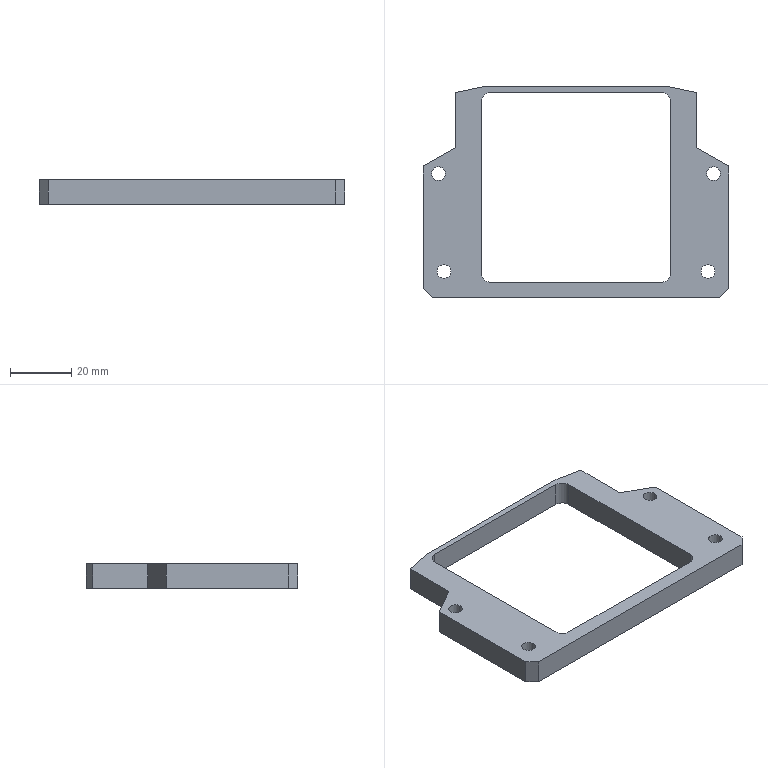Part | NX | 1 solid | 34 faces | box 100 x 69 x 8 mm | volume 19281 mm3 | plane 22 | cylinder 12 | commonest cylinder face diameters 4.5 x4 6 x4 8 x4
STEP:
#1=CARTESIAN_POINT('',(513.677,158.79,8.));
#2=VERTEX_POINT('',#1);
#3=CARTESIAN_POINT('',(515.927,158.79,8.));
#4=DIRECTION('',(0.,0.,-1.));
#5=DIRECTION('',(-1.,0.,0.));
#6=AXIS2_PLACEMENT_3D('',#3,#4,#5);
#7=CIRCLE('',#6,2.25);
#8=EDGE_CURVE('',#2,#2,#7,.T.);
#9=ORIENTED_EDGE('',*,*,#8,.F.);
#10=EDGE_LOOP('',(#9));
#11=FACE_BOUND('',#10,.T.);
#12=CARTESIAN_POINT('',(513.677,158.79,4.6));
#13=VERTEX_POINT('',#12);
#14=CARTESIAN_POINT('',(515.927,158.79,4.6));
#15=DIRECTION('',(0.,0.,1.));
#16=DIRECTION('',(-1.,0.,0.));
#17=AXIS2_PLACEMENT_3D('',#14,#15,#16);
#18=CIRCLE('',#17,2.25);
#19=EDGE_CURVE('',#13,#13,#18,.T.);
#20=ORIENTED_EDGE('',*,*,#19,.F.);
#21=EDGE_LOOP('',(#20));
#22=FACE_BOUND('',#21,.T.);
#23=CARTESIAN_POINT('',(515.927,158.79,8.));
#24=DIRECTION('',(0.,0.,-1.));
#25=DIRECTION('',(1.,0.,0.));
#26=AXIS2_PLACEMENT_3D('',#23,#24,#25);
#27=CYLINDRICAL_SURFACE('',#26,2.25);
#28=ADVANCED_FACE('',(#11,#22),#27,.F.);
#29=CARTESIAN_POINT('',(511.827,190.79,8.));
#30=VERTEX_POINT('',#29);
#31=CARTESIAN_POINT('',(514.077,190.79,8.));
#32=DIRECTION('',(0.,0.,-1.));
#33=DIRECTION('',(-1.,0.,0.));
#34=AXIS2_PLACEMENT_3D('',#31,#32,#33);
#35=CIRCLE('',#34,2.25);
#36=EDGE_CURVE('',#30,#30,#35,.T.);
#37=ORIENTED_EDGE('',*,*,#36,.F.);
#38=EDGE_LOOP('',(#37));
#39=FACE_BOUND('',#38,.T.);
#40=CARTESIAN_POINT('',(511.827,190.79,4.6));
#41=VERTEX_POINT('',#40);
#42=CARTESIAN_POINT('',(514.077,190.79,4.6));
#43=DIRECTION('',(0.,0.,1.));
#44=DIRECTION('',(-1.,0.,0.));
#45=AXIS2_PLACEMENT_3D('',#42,#43,#44);
#46=CIRCLE('',#45,2.25);
#47=EDGE_CURVE('',#41,#41,#46,.T.);
#48=ORIENTED_EDGE('',*,*,#47,.F.);
#49=EDGE_LOOP('',(#48));
#50=FACE_BOUND('',#49,.T.);
#51=CARTESIAN_POINT('',(514.077,190.79,8.));
#52=DIRECTION('',(0.,0.,-1.));
#53=DIRECTION('',(1.,0.,0.));
#54=AXIS2_PLACEMENT_3D('',#51,#52,#53);
#55=CYLINDRICAL_SURFACE('',#54,2.25);
#56=ADVANCED_FACE('',(#39,#50),#55,.F.);
#57=CARTESIAN_POINT('',(599.977,158.79,8.));
#58=VERTEX_POINT('',#57);
#59=CARTESIAN_POINT('',(602.227,158.79,8.));
#60=DIRECTION('',(0.,0.,-1.));
#61=DIRECTION('',(-1.,0.,0.));
#62=AXIS2_PLACEMENT_3D('',#59,#60,#61);
#63=CIRCLE('',#62,2.25);
#64=EDGE_CURVE('',#58,#58,#63,.T.);
#65=ORIENTED_EDGE('',*,*,#64,.F.);
#66=EDGE_LOOP('',(#65));
#67=FACE_BOUND('',#66,.T.);
#68=CARTESIAN_POINT('',(599.977,158.79,4.6));
#69=VERTEX_POINT('',#68);
#70=CARTESIAN_POINT('',(602.227,158.79,4.6));
#71=DIRECTION('',(0.,0.,1.));
#72=DIRECTION('',(-1.,0.,0.));
#73=AXIS2_PLACEMENT_3D('',#70,#71,#72);
#74=CIRCLE('',#73,2.25);
#75=EDGE_CURVE('',#69,#69,#74,.T.);
#76=ORIENTED_EDGE('',*,*,#75,.F.);
#77=EDGE_LOOP('',(#76));
#78=FACE_BOUND('',#77,.T.);
#79=CARTESIAN_POINT('',(602.227,158.79,8.));
#80=DIRECTION('',(0.,0.,-1.));
#81=DIRECTION('',(1.,0.,0.));
#82=AXIS2_PLACEMENT_3D('',#79,#80,#81);
#83=CYLINDRICAL_SURFACE('',#82,2.25);
#84=ADVANCED_FACE('',(#67,#78),#83,.F.);
#85=CARTESIAN_POINT('',(511.927,158.79,0.));
#86=VERTEX_POINT('',#85);
#87=CARTESIAN_POINT('',(515.927,158.79,0.));
#88=DIRECTION('',(0.,0.,-1.));
#89=DIRECTION('',(-1.,0.,0.));
#90=AXIS2_PLACEMENT_3D('',#87,#88,#89);
#91=CIRCLE('',#90,4.);
#92=EDGE_CURVE('',#86,#86,#91,.T.);
#93=ORIENTED_EDGE('',*,*,#92,.F.);
#94=EDGE_LOOP('',(#93));
#95=FACE_BOUND('',#94,.T.);
#96=CARTESIAN_POINT('',(528.077,158.29,0.));
#97=VERTEX_POINT('',#96);
#98=CARTESIAN_POINT('',(528.077,214.29,0.));
#99=VERTEX_POINT('',#98);
#100=CARTESIAN_POINT('',(528.077,158.29,0.));
#101=DIRECTION('',(0.,1.,0.));
#102=VECTOR('',#101,1.);
#103=LINE('',#100,#102);
#104=EDGE_CURVE('',#97,#99,#103,.T.);
#105=ORIENTED_EDGE('',*,*,#104,.F.);
#106=CARTESIAN_POINT('',(531.077,155.29,0.));
#107=VERTEX_POINT('',#106);
#108=CARTESIAN_POINT('',(531.077,158.29,0.));
#109=DIRECTION('',(0.,0.,-1.));
#110=DIRECTION('',(1.,0.,0.));
#111=AXIS2_PLACEMENT_3D('',#108,#109,#110);
#112=CIRCLE('',#111,3.);
#113=EDGE_CURVE('',#107,#97,#112,.T.);
#114=ORIENTED_EDGE('',*,*,#113,.F.);
#115=CARTESIAN_POINT('',(587.077,155.29,0.));
#116=VERTEX_POINT('',#115);
#117=CARTESIAN_POINT('',(587.077,155.29,0.));
#118=DIRECTION('',(-1.,0.,0.));
#119=VECTOR('',#118,1.);
#120=LINE('',#117,#119);
#121=EDGE_CURVE('',#116,#107,#120,.T.);
#122=ORIENTED_EDGE('',*,*,#121,.F.);
#123=CARTESIAN_POINT('',(590.077,158.29,0.));
#124=VERTEX_POINT('',#123);
#125=CARTESIAN_POINT('',(587.077,158.29,0.));
#126=DIRECTION('',(0.,0.,-1.));
#127=DIRECTION('',(1.,0.,0.));
#128=AXIS2_PLACEMENT_3D('',#125,#126,#127);
#129=CIRCLE('',#128,3.);
#130=EDGE_CURVE('',#124,#116,#129,.T.);
#131=ORIENTED_EDGE('',*,*,#130,.F.);
#132=CARTESIAN_POINT('',(590.077,214.29,0.));
#133=VERTEX_POINT('',#132);
#134=CARTESIAN_POINT('',(590.077,214.29,0.));
#135=DIRECTION('',(0.,-1.,0.));
#136=VECTOR('',#135,1.);
#137=LINE('',#134,#136);
#138=EDGE_CURVE('',#133,#124,#137,.T.);
#139=ORIENTED_EDGE('',*,*,#138,.F.);
#140=CARTESIAN_POINT('',(587.077,217.29,0.));
#141=VERTEX_POINT('',#140);
#142=CARTESIAN_POINT('',(587.077,214.29,0.));
#143=DIRECTION('',(0.,0.,-1.));
#144=DIRECTION('',(1.,0.,0.));
#145=AXIS2_PLACEMENT_3D('',#142,#143,#144);
#146=CIRCLE('',#145,3.);
#147=EDGE_CURVE('',#141,#133,#146,.T.);
#148=ORIENTED_EDGE('',*,*,#147,.F.);
#149=CARTESIAN_POINT('',(531.077,217.29,0.));
#150=VERTEX_POINT('',#149);
#151=CARTESIAN_POINT('',(531.077,217.29,0.));
#152=DIRECTION('',(1.,0.,0.));
#153=VECTOR('',#152,1.);
#154=LINE('',#151,#153);
#155=EDGE_CURVE('',#150,#141,#154,.T.);
#156=ORIENTED_EDGE('',*,*,#155,.F.);
#157=CARTESIAN_POINT('',(531.077,214.29,0.));
#158=DIRECTION('',(0.,0.,-1.));
#159=DIRECTION('',(1.,0.,0.));
#160=AXIS2_PLACEMENT_3D('',#157,#158,#159);
#161=CIRCLE('',#160,3.);
#162=EDGE_CURVE('',#99,#150,#161,.T.);
#163=ORIENTED_EDGE('',*,*,#162,.F.);
#164=EDGE_LOOP('',(#105,#114,#122,#131,#139,#148,#156,#163));
#165=FACE_BOUND('',#164,.T.);
#166=CARTESIAN_POINT('',(589.077,219.29,0.));
#167=VERTEX_POINT('',#166);
#168=CARTESIAN_POINT('',(529.077,219.29,0.));
#169=VERTEX_POINT('',#168);
#170=CARTESIAN_POINT('',(589.077,219.29,0.));
#171=DIRECTION('',(-1.,0.,0.));
#172=VECTOR('',#171,1.);
#173=LINE('',#170,#172);
#174=EDGE_CURVE('',#167,#169,#173,.T.);
#175=ORIENTED_EDGE('',*,*,#174,.F.);
#176=CARTESIAN_POINT('',(598.577,217.29,0.));
#177=VERTEX_POINT('',#176);
#178=CARTESIAN_POINT('',(598.577,217.29,0.));
#179=DIRECTION('',(-0.9785,0.206,0.));
#180=VECTOR('',#179,1.);
#181=LINE('',#178,#180);
#182=EDGE_CURVE('',#177,#167,#181,.T.);
#183=ORIENTED_EDGE('',*,*,#182,.F.);
#184=CARTESIAN_POINT('',(598.577,199.29,0.));
#185=VERTEX_POINT('',#184);
#186=CARTESIAN_POINT('',(598.577,199.29,0.));
#187=DIRECTION('',(0.,1.,0.));
#188=VECTOR('',#187,1.);
#189=LINE('',#186,#188);
#190=EDGE_CURVE('',#185,#177,#189,.T.);
#191=ORIENTED_EDGE('',*,*,#190,.F.);
#192=CARTESIAN_POINT('',(609.077,193.29,0.));
#193=VERTEX_POINT('',#192);
#194=CARTESIAN_POINT('',(609.077,193.29,0.));
#195=DIRECTION('',(-0.8682,0.4961,0.));
#196=VECTOR('',#195,1.);
#197=LINE('',#194,#196);
#198=EDGE_CURVE('',#193,#185,#197,.T.);
#199=ORIENTED_EDGE('',*,*,#198,.F.);
#200=CARTESIAN_POINT('',(609.077,153.29,0.));
#201=VERTEX_POINT('',#200);
#202=CARTESIAN_POINT('',(609.077,153.29,0.));
#203=DIRECTION('',(0.,1.,0.));
#204=VECTOR('',#203,1.);
#205=LINE('',#202,#204);
#206=EDGE_CURVE('',#201,#193,#205,.T.);
#207=ORIENTED_EDGE('',*,*,#206,.F.);
#208=CARTESIAN_POINT('',(606.077,150.29,0.));
#209=VERTEX_POINT('',#208);
#210=CARTESIAN_POINT('',(606.077,150.29,0.));
#211=DIRECTION('',(0.7071,0.7071,0.));
#212=VECTOR('',#211,1.);
#213=LINE('',#210,#212);
#214=EDGE_CURVE('',#209,#201,#213,.T.);
#215=ORIENTED_EDGE('',*,*,#214,.F.);
#216=CARTESIAN_POINT('',(512.077,150.29,0.));
#217=VERTEX_POINT('',#216);
#218=CARTESIAN_POINT('',(512.077,150.29,0.));
#219=DIRECTION('',(1.,0.,0.));
#220=VECTOR('',#219,1.);
#221=LINE('',#218,#220);
#222=EDGE_CURVE('',#217,#209,#221,.T.);
#223=ORIENTED_EDGE('',*,*,#222,.F.);
#224=CARTESIAN_POINT('',(509.077,153.29,0.));
#225=VERTEX_POINT('',#224);
#226=CARTESIAN_POINT('',(509.077,153.29,0.));
#227=DIRECTION('',(0.7071,-0.7071,0.));
#228=VECTOR('',#227,1.);
#229=LINE('',#226,#228);
#230=EDGE_CURVE('',#225,#217,#229,.T.);
#231=ORIENTED_EDGE('',*,*,#230,.F.);
#232=CARTESIAN_POINT('',(509.077,193.29,0.));
#233=VERTEX_POINT('',#232);
#234=CARTESIAN_POINT('',(509.077,193.29,0.));
#235=DIRECTION('',(0.,-1.,0.));
#236=VECTOR('',#235,1.);
#237=LINE('',#234,#236);
#238=EDGE_CURVE('',#233,#225,#237,.T.);
#239=ORIENTED_EDGE('',*,*,#238,.F.);
#240=CARTESIAN_POINT('',(519.577,199.29,0.));
#241=VERTEX_POINT('',#240);
#242=CARTESIAN_POINT('',(519.577,199.29,0.));
#243=DIRECTION('',(-0.8682,-0.4961,0.));
#244=VECTOR('',#243,1.);
#245=LINE('',#242,#244);
#246=EDGE_CURVE('',#241,#233,#245,.T.);
#247=ORIENTED_EDGE('',*,*,#246,.F.);
#248=CARTESIAN_POINT('',(519.577,217.29,0.));
#249=VERTEX_POINT('',#248);
#250=CARTESIAN_POINT('',(519.577,217.29,0.));
#251=DIRECTION('',(0.,-1.,0.));
#252=VECTOR('',#251,1.);
#253=LINE('',#250,#252);
#254=EDGE_CURVE('',#249,#241,#253,.T.);
#255=ORIENTED_EDGE('',*,*,#254,.F.);
#256=CARTESIAN_POINT('',(529.077,219.29,0.));
#257=DIRECTION('',(-0.9785,-0.206,0.));
#258=VECTOR('',#257,1.);
#259=LINE('',#256,#258);
#260=EDGE_CURVE('',#169,#249,#259,.T.);
#261=ORIENTED_EDGE('',*,*,#260,.F.);
#262=EDGE_LOOP('',(#175,#183,#191,#199,#207,#215,#223,#231,#239,#247,#255,#261));
#263=FACE_BOUND('',#262,.T.);
#264=CARTESIAN_POINT('',(600.077,190.79,0.));
#265=VERTEX_POINT('',#264);
#266=CARTESIAN_POINT('',(604.077,190.79,0.));
#267=DIRECTION('',(0.,0.,1.));
#268=DIRECTION('',(-1.,0.,0.));
#269=AXIS2_PLACEMENT_3D('',#266,#267,#268);
#270=CIRCLE('',#269,4.);
#271=EDGE_CURVE('',#265,#265,#270,.T.);
#272=ORIENTED_EDGE('',*,*,#271,.T.);
#273=EDGE_LOOP('',(#272));
#274=FACE_BOUND('',#273,.T.);
#275=CARTESIAN_POINT('',(510.077,190.79,0.));
#276=VERTEX_POINT('',#275);
#277=CARTESIAN_POINT('',(514.077,190.79,0.));
#278=DIRECTION('',(0.,0.,-1.));
#279=DIRECTION('',(-1.,0.,0.));
#280=AXIS2_PLACEMENT_3D('',#277,#278,#279);
#281=CIRCLE('',#280,4.);
#282=EDGE_CURVE('',#276,#276,#281,.T.);
#283=ORIENTED_EDGE('',*,*,#282,.F.);
#284=EDGE_LOOP('',(#283));
#285=FACE_BOUND('',#284,.T.);
#286=CARTESIAN_POINT('',(598.227,158.79,0.));
#287=VERTEX_POINT('',#286);
#288=CARTESIAN_POINT('',(602.227,158.79,0.));
#289=DIRECTION('',(0.,0.,-1.));
#290=DIRECTION('',(-1.,0.,0.));
#291=AXIS2_PLACEMENT_3D('',#288,#289,#290);
#292=CIRCLE('',#291,4.);
#293=EDGE_CURVE('',#287,#287,#292,.T.);
#294=ORIENTED_EDGE('',*,*,#293,.F.);
#295=EDGE_LOOP('',(#294));
#296=FACE_BOUND('',#295,.T.);
#297=CARTESIAN_POINT('',(604.077,190.79,0.));
#298=DIRECTION('',(0.,0.,1.));
#299=DIRECTION('',(-1.,0.,0.));
#300=AXIS2_PLACEMENT_3D('',#297,#298,#299);
#301=PLANE('',#300);
#302=ADVANCED_FACE('',(#95,#165,#263,#274,#285,#296),#301,.F.);
#303=ORIENTED_EDGE('',*,*,#104,.T.);
#304=CARTESIAN_POINT('',(528.077,214.29,8.));
#305=VERTEX_POINT('',#304);
#306=CARTESIAN_POINT('',(528.077,214.29,8.));
#307=DIRECTION('',(0.,0.,-1.));
#308=VECTOR('',#307,1.);
#309=LINE('',#306,#308);
#310=EDGE_CURVE('',#305,#99,#309,.T.);
#311=ORIENTED_EDGE('',*,*,#310,.F.);
#312=CARTESIAN_POINT('',(528.077,158.29,8.));
#313=VERTEX_POINT('',#312);
#314=CARTESIAN_POINT('',(528.077,158.29,8.));
#315=DIRECTION('',(0.,1.,0.));
#316=VECTOR('',#315,1.);
#317=LINE('',#314,#316);
#318=EDGE_CURVE('',#313,#305,#317,.T.);
#319=ORIENTED_EDGE('',*,*,#318,.F.);
#320=CARTESIAN_POINT('',(528.077,158.29,8.));
#321=DIRECTION('',(0.,0.,-1.));
#322=VECTOR('',#321,1.);
#323=LINE('',#320,#322);
#324=EDGE_CURVE('',#313,#97,#323,.T.);
#325=ORIENTED_EDGE('',*,*,#324,.T.);
#326=EDGE_LOOP('',(#303,#311,#319,#325));
#327=FACE_OUTER_BOUND('',#326,.T.);
#328=CARTESIAN_POINT('',(528.077,158.29,8.));
#329=DIRECTION('',(-1.,0.,0.));
#330=DIRECTION('',(0.,0.,-1.));
#331=AXIS2_PLACEMENT_3D('',#328,#329,#330);
#332=PLANE('',#331);
#333=ADVANCED_FACE('',(#327),#332,.F.);
#334=ORIENTED_EDGE('',*,*,#162,.T.);
#335=CARTESIAN_POINT('',(531.077,217.29,8.));
#336=VERTEX_POINT('',#335);
#337=CARTESIAN_POINT('',(531.077,217.29,8.));
#338=DIRECTION('',(0.,0.,-1.));
#339=VECTOR('',#338,1.);
#340=LINE('',#337,#339);
#341=EDGE_CURVE('',#336,#150,#340,.T.);
#342=ORIENTED_EDGE('',*,*,#341,.F.);
#343=CARTESIAN_POINT('',(531.077,214.29,8.));
#344=DIRECTION('',(0.,0.,-1.));
#345=DIRECTION('',(1.,0.,0.));
#346=AXIS2_PLACEMENT_3D('',#343,#344,#345);
#347=CIRCLE('',#346,3.);
#348=EDGE_CURVE('',#305,#336,#347,.T.);
#349=ORIENTED_EDGE('',*,*,#348,.F.);
#350=ORIENTED_EDGE('',*,*,#310,.T.);
#351=EDGE_LOOP('',(#334,#342,#349,#350));
#352=FACE_OUTER_BOUND('',#351,.T.);
#353=CARTESIAN_POINT('',(531.077,214.29,8.));
#354=DIRECTION('',(0.,0.,-1.));
#355=DIRECTION('',(1.,0.,0.));
#356=AXIS2_PLACEMENT_3D('',#353,#354,#355);
#357=CYLINDRICAL_SURFACE('',#356,3.);
#358=ADVANCED_FACE('',(#352),#357,.F.);
#359=ORIENTED_EDGE('',*,*,#155,.T.);
#360=CARTESIAN_POINT('',(587.077,217.29,8.));
#361=VERTEX_POINT('',#360);
#362=CARTESIAN_POINT('',(587.077,217.29,8.));
#363=DIRECTION('',(0.,0.,-1.));
#364=VECTOR('',#363,1.);
#365=LINE('',#362,#364);
#366=EDGE_CURVE('',#361,#141,#365,.T.);
#367=ORIENTED_EDGE('',*,*,#366,.F.);
#368=CARTESIAN_POINT('',(531.077,217.29,8.));
#369=DIRECTION('',(1.,0.,0.));
#370=VECTOR('',#369,1.);
#371=LINE('',#368,#370);
#372=EDGE_CURVE('',#336,#361,#371,.T.);
#373=ORIENTED_EDGE('',*,*,#372,.F.);
#374=ORIENTED_EDGE('',*,*,#341,.T.);
#375=EDGE_LOOP('',(#359,#367,#373,#374));
#376=FACE_OUTER_BOUND('',#375,.T.);
#377=CARTESIAN_POINT('',(531.077,217.29,8.));
#378=DIRECTION('',(0.,1.,0.));
#379=DIRECTION('',(0.,0.,-1.));
#380=AXIS2_PLACEMENT_3D('',#377,#378,#379);
#381=PLANE('',#380);
#382=ADVANCED_FACE('',(#376),#381,.F.);
#383=ORIENTED_EDGE('',*,*,#147,.T.);
#384=CARTESIAN_POINT('',(590.077,214.29,8.));
#385=VERTEX_POINT('',#384);
#386=CARTESIAN_POINT('',(590.077,214.29,8.));
#387=DIRECTION('',(0.,0.,-1.));
#388=VECTOR('',#387,1.);
#389=LINE('',#386,#388);
#390=EDGE_CURVE('',#385,#133,#389,.T.);
#391=ORIENTED_EDGE('',*,*,#390,.F.);
#392=CARTESIAN_POINT('',(587.077,214.29,8.));
#393=DIRECTION('',(0.,0.,-1.));
#394=DIRECTION('',(1.,0.,0.));
#395=AXIS2_PLACEMENT_3D('',#392,#393,#394);
#396=CIRCLE('',#395,3.);
#397=EDGE_CURVE('',#361,#385,#396,.T.);
#398=ORIENTED_EDGE('',*,*,#397,.F.);
#399=ORIENTED_EDGE('',*,*,#366,.T.);
#400=EDGE_LOOP('',(#383,#391,#398,#399));
#401=FACE_OUTER_BOUND('',#400,.T.);
#402=CARTESIAN_POINT('',(587.077,214.29,8.));
#403=DIRECTION('',(0.,0.,-1.));
#404=DIRECTION('',(1.,0.,0.));
#405=AXIS2_PLACEMENT_3D('',#402,#403,#404);
#406=CYLINDRICAL_SURFACE('',#405,3.);
#407=ADVANCED_FACE('',(#401),#406,.F.);
#408=ORIENTED_EDGE('',*,*,#138,.T.);
#409=CARTESIAN_POINT('',(590.077,158.29,8.));
#410=VERTEX_POINT('',#409);
#411=CARTESIAN_POINT('',(590.077,158.29,8.));
#412=DIRECTION('',(0.,0.,-1.));
#413=VECTOR('',#412,1.);
#414=LINE('',#411,#413);
#415=EDGE_CURVE('',#410,#124,#414,.T.);
#416=ORIENTED_EDGE('',*,*,#415,.F.);
#417=CARTESIAN_POINT('',(590.077,214.29,8.));
#418=DIRECTION('',(0.,-1.,0.));
#419=VECTOR('',#418,1.);
#420=LINE('',#417,#419);
#421=EDGE_CURVE('',#385,#410,#420,.T.);
#422=ORIENTED_EDGE('',*,*,#421,.F.);
#423=ORIENTED_EDGE('',*,*,#390,.T.);
#424=EDGE_LOOP('',(#408,#416,#422,#423));
#425=FACE_OUTER_BOUND('',#424,.T.);
#426=CARTESIAN_POINT('',(590.077,214.29,8.));
#427=DIRECTION('',(1.,0.,0.));
#428=DIRECTION('',(0.,0.,1.));
#429=AXIS2_PLACEMENT_3D('',#426,#427,#428);
#430=PLANE('',#429);
#431=ADVANCED_FACE('',(#425),#430,.F.);
#432=ORIENTED_EDGE('',*,*,#130,.T.);
#433=CARTESIAN_POINT('',(587.077,155.29,8.));
#434=VERTEX_POINT('',#433);
#435=CARTESIAN_POINT('',(587.077,155.29,8.));
#436=DIRECTION('',(0.,0.,-1.));
#437=VECTOR('',#436,1.);
#438=LINE('',#435,#437);
#439=EDGE_CURVE('',#434,#116,#438,.T.);
#440=ORIENTED_EDGE('',*,*,#439,.F.);
#441=CARTESIAN_POINT('',(587.077,158.29,8.));
#442=DIRECTION('',(0.,0.,-1.));
#443=DIRECTION('',(1.,0.,0.));
#444=AXIS2_PLACEMENT_3D('',#441,#442,#443);
#445=CIRCLE('',#444,3.);
#446=EDGE_CURVE('',#410,#434,#445,.T.);
#447=ORIENTED_EDGE('',*,*,#446,.F.);
#448=ORIENTED_EDGE('',*,*,#415,.T.);
#449=EDGE_LOOP('',(#432,#440,#447,#448));
#450=FACE_OUTER_BOUND('',#449,.T.);
#451=CARTESIAN_POINT('',(587.077,158.29,8.));
#452=DIRECTION('',(0.,0.,-1.));
#453=DIRECTION('',(1.,0.,0.));
#454=AXIS2_PLACEMENT_3D('',#451,#452,#453);
#455=CYLINDRICAL_SURFACE('',#454,3.);
#456=ADVANCED_FACE('',(#450),#455,.F.);
#457=ORIENTED_EDGE('',*,*,#121,.T.);
#458=CARTESIAN_POINT('',(531.077,155.29,8.));
#459=VERTEX_POINT('',#458);
#460=CARTESIAN_POINT('',(531.077,155.29,8.));
#461=DIRECTION('',(0.,0.,-1.));
#462=VECTOR('',#461,1.);
#463=LINE('',#460,#462);
#464=EDGE_CURVE('',#459,#107,#463,.T.);
#465=ORIENTED_EDGE('',*,*,#464,.F.);
#466=CARTESIAN_POINT('',(587.077,155.29,8.));
#467=DIRECTION('',(-1.,0.,0.));
#468=VECTOR('',#467,1.);
#469=LINE('',#466,#468);
#470=EDGE_CURVE('',#434,#459,#469,.T.);
#471=ORIENTED_EDGE('',*,*,#470,.F.);
#472=ORIENTED_EDGE('',*,*,#439,.T.);
#473=EDGE_LOOP('',(#457,#465,#471,#472));
#474=FACE_OUTER_BOUND('',#473,.T.);
#475=CARTESIAN_POINT('',(587.077,155.29,8.));
#476=DIRECTION('',(0.,-1.,0.));
#477=DIRECTION('',(0.,0.,1.));
#478=AXIS2_PLACEMENT_3D('',#475,#476,#477);
#479=PLANE('',#478);
#480=ADVANCED_FACE('',(#474),#479,.F.);
#481=ORIENTED_EDGE('',*,*,#174,.T.);
#482=CARTESIAN_POINT('',(529.077,219.29,8.));
#483=VERTEX_POINT('',#482);
#484=CARTESIAN_POINT('',(529.077,219.29,8.));
#485=DIRECTION('',(0.,0.,-1.));
#486=VECTOR('',#485,1.);
#487=LINE('',#484,#486);
#488=EDGE_CURVE('',#483,#169,#487,.T.);
#489=ORIENTED_EDGE('',*,*,#488,.F.);
#490=CARTESIAN_POINT('',(589.077,219.29,8.));
#491=VERTEX_POINT('',#490);
#492=CARTESIAN_POINT('',(589.077,219.29,8.));
#493=DIRECTION('',(-1.,0.,0.));
#494=VECTOR('',#493,1.);
#495=LINE('',#492,#494);
#496=EDGE_CURVE('',#491,#483,#495,.T.);
#497=ORIENTED_EDGE('',*,*,#496,.F.);
#498=CARTESIAN_POINT('',(589.077,219.29,8.));
#499=DIRECTION('',(0.,0.,-1.));
#500=VECTOR('',#499,1.);
#501=LINE('',#498,#500);
#502=EDGE_CURVE('',#491,#167,#501,.T.);
#503=ORIENTED_EDGE('',*,*,#502,.T.);
#504=EDGE_LOOP('',(#481,#489,#497,#503));
#505=FACE_OUTER_BOUND('',#504,.T.);
#506=CARTESIAN_POINT('',(589.077,219.29,8.));
#507=DIRECTION('',(0.,-1.,0.));
#508=DIRECTION('',(-1.,0.,0.));
#509=AXIS2_PLACEMENT_3D('',#506,#507,#508);
#510=PLANE('',#509);
#511=ADVANCED_FACE('',(#505),#510,.F.);
#512=ORIENTED_EDGE('',*,*,#260,.T.);
#513=CARTESIAN_POINT('',(519.577,217.29,8.));
#514=VERTEX_POINT('',#513);
#515=CARTESIAN_POINT('',(519.577,217.29,8.));
#516=DIRECTION('',(0.,0.,-1.));
#517=VECTOR('',#516,1.);
#518=LINE('',#515,#517);
#519=EDGE_CURVE('',#514,#249,#518,.T.);
#520=ORIENTED_EDGE('',*,*,#519,.F.);
#521=CARTESIAN_POINT('',(529.077,219.29,8.));
#522=DIRECTION('',(-0.9785,-0.206,0.));
#523=VECTOR('',#522,1.);
#524=LINE('',#521,#523);
#525=EDGE_CURVE('',#483,#514,#524,.T.);
#526=ORIENTED_EDGE('',*,*,#525,.F.);
#527=ORIENTED_EDGE('',*,*,#488,.T.);
#528=EDGE_LOOP('',(#512,#520,#526,#527));
#529=FACE_OUTER_BOUND('',#528,.T.);
#530=CARTESIAN_POINT('',(529.077,219.29,8.));
#531=DIRECTION('',(0.206,-0.9785,0.));
#532=DIRECTION('',(-0.9785,-0.206,0.));
#533=AXIS2_PLACEMENT_3D('',#530,#531,#532);
#534=PLANE('',#533);
#535=ADVANCED_FACE('',(#529),#534,.F.);
#536=ORIENTED_EDGE('',*,*,#254,.T.);
#537=CARTESIAN_POINT('',(519.577,199.29,8.));
#538=VERTEX_POINT('',#537);
#539=CARTESIAN_POINT('',(519.577,199.29,8.));
#540=DIRECTION('',(0.,0.,-1.));
#541=VECTOR('',#540,1.);
#542=LINE('',#539,#541);
#543=EDGE_CURVE('',#538,#241,#542,.T.);
#544=ORIENTED_EDGE('',*,*,#543,.F.);
#545=CARTESIAN_POINT('',(519.577,217.29,8.));
#546=DIRECTION('',(0.,-1.,0.));
#547=VECTOR('',#546,1.);
#548=LINE('',#545,#547);
#549=EDGE_CURVE('',#514,#538,#548,.T.);
#550=ORIENTED_EDGE('',*,*,#549,.F.);
#551=ORIENTED_EDGE('',*,*,#519,.T.);
#552=EDGE_LOOP('',(#536,#544,#550,#551));
#553=FACE_OUTER_BOUND('',#552,.T.);
#554=CARTESIAN_POINT('',(519.577,217.29,8.));
#555=DIRECTION('',(1.,0.,0.));
#556=DIRECTION('',(0.,0.,1.));
#557=AXIS2_PLACEMENT_3D('',#554,#555,#556);
#558=PLANE('',#557);
#559=ADVANCED_FACE('',(#553),#558,.F.);
#560=ORIENTED_EDGE('',*,*,#246,.T.);
#561=CARTESIAN_POINT('',(509.077,193.29,8.));
#562=VERTEX_POINT('',#561);
#563=CARTESIAN_POINT('',(509.077,193.29,8.));
#564=DIRECTION('',(0.,0.,-1.));
#565=VECTOR('',#564,1.);
#566=LINE('',#563,#565);
#567=EDGE_CURVE('',#562,#233,#566,.T.);
#568=ORIENTED_EDGE('',*,*,#567,.F.);
#569=CARTESIAN_POINT('',(519.577,199.29,8.));
#570=DIRECTION('',(-0.8682,-0.4961,0.));
#571=VECTOR('',#570,1.);
#572=LINE('',#569,#571);
#573=EDGE_CURVE('',#538,#562,#572,.T.);
#574=ORIENTED_EDGE('',*,*,#573,.F.);
#575=ORIENTED_EDGE('',*,*,#543,.T.);
#576=EDGE_LOOP('',(#560,#568,#574,#575));
#577=FACE_OUTER_BOUND('',#576,.T.);
#578=CARTESIAN_POINT('',(519.577,199.29,8.));
#579=DIRECTION('',(0.4961,-0.8682,0.));
#580=DIRECTION('',(-0.8682,-0.4961,0.));
#581=AXIS2_PLACEMENT_3D('',#578,#579,#580);
#582=PLANE('',#581);
#583=ADVANCED_FACE('',(#577),#582,.F.);
#584=ORIENTED_EDGE('',*,*,#238,.T.);
#585=CARTESIAN_POINT('',(509.077,153.29,8.));
#586=VERTEX_POINT('',#585);
#587=CARTESIAN_POINT('',(509.077,153.29,8.));
#588=DIRECTION('',(0.,0.,-1.));
#589=VECTOR('',#588,1.);
#590=LINE('',#587,#589);
#591=EDGE_CURVE('',#586,#225,#590,.T.);
#592=ORIENTED_EDGE('',*,*,#591,.F.);
#593=CARTESIAN_POINT('',(509.077,193.29,8.));
#594=DIRECTION('',(0.,-1.,0.));
#595=VECTOR('',#594,1.);
#596=LINE('',#593,#595);
#597=EDGE_CURVE('',#562,#586,#596,.T.);
#598=ORIENTED_EDGE('',*,*,#597,.F.);
#599=ORIENTED_EDGE('',*,*,#567,.T.);
#600=EDGE_LOOP('',(#584,#592,#598,#599));
#601=FACE_OUTER_BOUND('',#600,.T.);
#602=CARTESIAN_POINT('',(509.077,193.29,8.));
#603=DIRECTION('',(1.,0.,0.));
#604=DIRECTION('',(0.,0.,1.));
#605=AXIS2_PLACEMENT_3D('',#602,#603,#604);
#606=PLANE('',#605);
#607=ADVANCED_FACE('',(#601),#606,.F.);
#608=ORIENTED_EDGE('',*,*,#230,.T.);
#609=CARTESIAN_POINT('',(512.077,150.29,8.));
#610=VERTEX_POINT('',#609);
#611=CARTESIAN_POINT('',(512.077,150.29,8.));
#612=DIRECTION('',(0.,0.,-1.));
#613=VECTOR('',#612,1.);
#614=LINE('',#611,#613);
#615=EDGE_CURVE('',#610,#217,#614,.T.);
#616=ORIENTED_EDGE('',*,*,#615,.F.);
#617=CARTESIAN_POINT('',(509.077,153.29,8.));
#618=DIRECTION('',(0.7071,-0.7071,0.));
#619=VECTOR('',#618,1.);
#620=LINE('',#617,#619);
#621=EDGE_CURVE('',#586,#610,#620,.T.);
#622=ORIENTED_EDGE('',*,*,#621,.F.);
#623=ORIENTED_EDGE('',*,*,#591,.T.);
#624=EDGE_LOOP('',(#608,#616,#622,#623));
#625=FACE_OUTER_BOUND('',#624,.T.);
#626=CARTESIAN_POINT('',(509.077,153.29,8.));
#627=DIRECTION('',(0.7071,0.7071,0.));
#628=DIRECTION('',(0.7071,-0.7071,0.));
#629=AXIS2_PLACEMENT_3D('',#626,#627,#628);
#630=PLANE('',#629);
#631=ADVANCED_FACE('',(#625),#630,.F.);
#632=ORIENTED_EDGE('',*,*,#222,.T.);
#633=CARTESIAN_POINT('',(606.077,150.29,8.));
#634=VERTEX_POINT('',#633);
#635=CARTESIAN_POINT('',(606.077,150.29,8.));
#636=DIRECTION('',(0.,0.,-1.));
#637=VECTOR('',#636,1.);
#638=LINE('',#635,#637);
#639=EDGE_CURVE('',#634,#209,#638,.T.);
#640=ORIENTED_EDGE('',*,*,#639,.F.);
#641=CARTESIAN_POINT('',(512.077,150.29,8.));
#642=DIRECTION('',(1.,0.,0.));
#643=VECTOR('',#642,1.);
#644=LINE('',#641,#643);
#645=EDGE_CURVE('',#610,#634,#644,.T.);
#646=ORIENTED_EDGE('',*,*,#645,.F.);
#647=ORIENTED_EDGE('',*,*,#615,.T.);
#648=EDGE_LOOP('',(#632,#640,#646,#647));
#649=FACE_OUTER_BOUND('',#648,.T.);
#650=CARTESIAN_POINT('',(512.077,150.29,8.));
#651=DIRECTION('',(0.,1.,0.));
#652=DIRECTION('',(0.,0.,-1.));
#653=AXIS2_PLACEMENT_3D('',#650,#651,#652);
#654=PLANE('',#653);
#655=ADVANCED_FACE('',(#649),#654,.F.);
#656=ORIENTED_EDGE('',*,*,#214,.T.);
#657=CARTESIAN_POINT('',(609.077,153.29,8.));
#658=VERTEX_POINT('',#657);
#659=CARTESIAN_POINT('',(609.077,153.29,8.));
#660=DIRECTION('',(0.,0.,-1.));
#661=VECTOR('',#660,1.);
#662=LINE('',#659,#661);
#663=EDGE_CURVE('',#658,#201,#662,.T.);
#664=ORIENTED_EDGE('',*,*,#663,.F.);
#665=CARTESIAN_POINT('',(606.077,150.29,8.));
#666=DIRECTION('',(0.7071,0.7071,0.));
#667=VECTOR('',#666,1.);
#668=LINE('',#665,#667);
#669=EDGE_CURVE('',#634,#658,#668,.T.);
#670=ORIENTED_EDGE('',*,*,#669,.F.);
#671=ORIENTED_EDGE('',*,*,#639,.T.);
#672=EDGE_LOOP('',(#656,#664,#670,#671));
#673=FACE_OUTER_BOUND('',#672,.T.);
#674=CARTESIAN_POINT('',(606.077,150.29,8.));
#675=DIRECTION('',(-0.7071,0.7071,0.));
#676=DIRECTION('',(0.7071,0.7071,0.));
#677=AXIS2_PLACEMENT_3D('',#674,#675,#676);
#678=PLANE('',#677);
#679=ADVANCED_FACE('',(#673),#678,.F.);
#680=ORIENTED_EDGE('',*,*,#206,.T.);
#681=CARTESIAN_POINT('',(609.077,193.29,8.));
#682=VERTEX_POINT('',#681);
#683=CARTESIAN_POINT('',(609.077,193.29,8.));
#684=DIRECTION('',(0.,0.,-1.));
#685=VECTOR('',#684,1.);
#686=LINE('',#683,#685);
#687=EDGE_CURVE('',#682,#193,#686,.T.);
#688=ORIENTED_EDGE('',*,*,#687,.F.);
#689=CARTESIAN_POINT('',(609.077,153.29,8.));
#690=DIRECTION('',(0.,1.,0.));
#691=VECTOR('',#690,1.);
#692=LINE('',#689,#691);
#693=EDGE_CURVE('',#658,#682,#692,.T.);
#694=ORIENTED_EDGE('',*,*,#693,.F.);
#695=ORIENTED_EDGE('',*,*,#663,.T.);
#696=EDGE_LOOP('',(#680,#688,#694,#695));
#697=FACE_OUTER_BOUND('',#696,.T.);
#698=CARTESIAN_POINT('',(609.077,153.29,8.));
#699=DIRECTION('',(-1.,0.,0.));
#700=DIRECTION('',(0.,0.,-1.));
#701=AXIS2_PLACEMENT_3D('',#698,#699,#700);
#702=PLANE('',#701);
#703=ADVANCED_FACE('',(#697),#702,.F.);
#704=ORIENTED_EDGE('',*,*,#198,.T.);
#705=CARTESIAN_POINT('',(598.577,199.29,8.));
#706=VERTEX_POINT('',#705);
#707=CARTESIAN_POINT('',(598.577,199.29,8.));
#708=DIRECTION('',(0.,0.,-1.));
#709=VECTOR('',#708,1.);
#710=LINE('',#707,#709);
#711=EDGE_CURVE('',#706,#185,#710,.T.);
#712=ORIENTED_EDGE('',*,*,#711,.F.);
#713=CARTESIAN_POINT('',(609.077,193.29,8.));
#714=DIRECTION('',(-0.8682,0.4961,0.));
#715=VECTOR('',#714,1.);
#716=LINE('',#713,#715);
#717=EDGE_CURVE('',#682,#706,#716,.T.);
#718=ORIENTED_EDGE('',*,*,#717,.F.);
#719=ORIENTED_EDGE('',*,*,#687,.T.);
#720=EDGE_LOOP('',(#704,#712,#718,#719));
#721=FACE_OUTER_BOUND('',#720,.T.);
#722=CARTESIAN_POINT('',(609.077,193.29,8.));
#723=DIRECTION('',(-0.4961,-0.8682,0.));
#724=DIRECTION('',(-0.8682,0.4961,0.));
#725=AXIS2_PLACEMENT_3D('',#722,#723,#724);
#726=PLANE('',#725);
#727=ADVANCED_FACE('',(#721),#726,.F.);
#728=ORIENTED_EDGE('',*,*,#190,.T.);
#729=CARTESIAN_POINT('',(598.577,217.29,8.));
#730=VERTEX_POINT('',#729);
#731=CARTESIAN_POINT('',(598.577,217.29,8.));
#732=DIRECTION('',(0.,0.,-1.));
#733=VECTOR('',#732,1.);
#734=LINE('',#731,#733);
#735=EDGE_CURVE('',#730,#177,#734,.T.);
#736=ORIENTED_EDGE('',*,*,#735,.F.);
#737=CARTESIAN_POINT('',(598.577,199.29,8.));
#738=DIRECTION('',(0.,1.,0.));
#739=VECTOR('',#738,1.);
#740=LINE('',#737,#739);
#741=EDGE_CURVE('',#706,#730,#740,.T.);
#742=ORIENTED_EDGE('',*,*,#741,.F.);
#743=ORIENTED_EDGE('',*,*,#711,.T.);
#744=EDGE_LOOP('',(#728,#736,#742,#743));
#745=FACE_OUTER_BOUND('',#744,.T.);
#746=CARTESIAN_POINT('',(598.577,199.29,8.));
#747=DIRECTION('',(-1.,0.,0.));
#748=DIRECTION('',(0.,0.,-1.));
#749=AXIS2_PLACEMENT_3D('',#746,#747,#748);
#750=PLANE('',#749);
#751=ADVANCED_FACE('',(#745),#750,.F.);
#752=ORIENTED_EDGE('',*,*,#113,.T.);
#753=ORIENTED_EDGE('',*,*,#324,.F.);
#754=CARTESIAN_POINT('',(531.077,158.29,8.));
#755=DIRECTION('',(0.,0.,-1.));
#756=DIRECTION('',(1.,0.,0.));
#757=AXIS2_PLACEMENT_3D('',#754,#755,#756);
#758=CIRCLE('',#757,3.);
#759=EDGE_CURVE('',#459,#313,#758,.T.);
#760=ORIENTED_EDGE('',*,*,#759,.F.);
#761=ORIENTED_EDGE('',*,*,#464,.T.);
#762=EDGE_LOOP('',(#752,#753,#760,#761));
#763=FACE_OUTER_BOUND('',#762,.T.);
#764=CARTESIAN_POINT('',(531.077,158.29,8.));
#765=DIRECTION('',(0.,0.,-1.));
#766=DIRECTION('',(1.,0.,0.));
#767=AXIS2_PLACEMENT_3D('',#764,#765,#766);
#768=CYLINDRICAL_SURFACE('',#767,3.);
#769=ADVANCED_FACE('',(#763),#768,.F.);
#770=CARTESIAN_POINT('',(606.327,190.79,4.6));
#771=VERTEX_POINT('',#770);
#772=CARTESIAN_POINT('',(604.077,190.79,4.6));
#773=DIRECTION('',(0.,0.,1.));
#774=DIRECTION('',(1.,0.,0.));
#775=AXIS2_PLACEMENT_3D('',#772,#773,#774);
#776=CIRCLE('',#775,2.25);
#777=EDGE_CURVE('',#771,#771,#776,.T.);
#778=ORIENTED_EDGE('',*,*,#777,.F.);
#779=EDGE_LOOP('',(#778));
#780=FACE_BOUND('',#779,.T.);
#781=CARTESIAN_POINT('',(601.827,190.79,8.));
#782=VERTEX_POINT('',#781);
#783=CARTESIAN_POINT('',(604.077,190.79,8.));
#784=DIRECTION('',(0.,0.,1.));
#785=DIRECTION('',(-1.,0.,0.));
#786=AXIS2_PLACEMENT_3D('',#783,#784,#785);
#787=CIRCLE('',#786,2.25);
#788=EDGE_CURVE('',#782,#782,#787,.T.);
#789=ORIENTED_EDGE('',*,*,#788,.T.);
#790=EDGE_LOOP('',(#789));
#791=FACE_BOUND('',#790,.T.);
#792=CARTESIAN_POINT('',(604.077,190.79,8.));
#793=DIRECTION('',(0.,0.,-1.));
#794=DIRECTION('',(1.,0.,0.));
#795=AXIS2_PLACEMENT_3D('',#792,#793,#794);
#796=CYLINDRICAL_SURFACE('',#795,2.25);
#797=ADVANCED_FACE('',(#780,#791),#796,.F.);
#798=ORIENTED_EDGE('',*,*,#182,.T.);
#799=ORIENTED_EDGE('',*,*,#502,.F.);
#800=CARTESIAN_POINT('',(598.577,217.29,8.));
#801=DIRECTION('',(-0.9785,0.206,0.));
#802=VECTOR('',#801,1.);
#803=LINE('',#800,#802);
#804=EDGE_CURVE('',#730,#491,#803,.T.);
#805=ORIENTED_EDGE('',*,*,#804,.F.);
#806=ORIENTED_EDGE('',*,*,#735,.T.);
#807=EDGE_LOOP('',(#798,#799,#805,#806));
#808=FACE_OUTER_BOUND('',#807,.T.);
#809=CARTESIAN_POINT('',(598.577,217.29,8.));
#810=DIRECTION('',(-0.206,-0.9785,0.));
#811=DIRECTION('',(-0.9785,0.206,0.));
#812=AXIS2_PLACEMENT_3D('',#809,#810,#811);
#813=PLANE('',#812);
#814=ADVANCED_FACE('',(#808),#813,.F.);
#815=ORIENTED_EDGE('',*,*,#496,.T.);
#816=ORIENTED_EDGE('',*,*,#525,.T.);
#817=ORIENTED_EDGE('',*,*,#549,.T.);
#818=ORIENTED_EDGE('',*,*,#573,.T.);
#819=ORIENTED_EDGE('',*,*,#597,.T.);
#820=ORIENTED_EDGE('',*,*,#621,.T.);
#821=ORIENTED_EDGE('',*,*,#645,.T.);
#822=ORIENTED_EDGE('',*,*,#669,.T.);
#823=ORIENTED_EDGE('',*,*,#693,.T.);
#824=ORIENTED_EDGE('',*,*,#717,.T.);
#825=ORIENTED_EDGE('',*,*,#741,.T.);
#826=ORIENTED_EDGE('',*,*,#804,.T.);
#827=EDGE_LOOP('',(#815,#816,#817,#818,#819,#820,#821,#822,#823,#824,#825,#826));
#828=FACE_BOUND('',#827,.T.);
#829=ORIENTED_EDGE('',*,*,#788,.F.);
#830=EDGE_LOOP('',(#829));
#831=FACE_BOUND('',#830,.T.);
#832=ORIENTED_EDGE('',*,*,#36,.T.);
#833=EDGE_LOOP('',(#832));
#834=FACE_BOUND('',#833,.T.);
#835=ORIENTED_EDGE('',*,*,#8,.T.);
#836=EDGE_LOOP('',(#835));
#837=FACE_BOUND('',#836,.T.);
#838=ORIENTED_EDGE('',*,*,#318,.T.);
#839=ORIENTED_EDGE('',*,*,#348,.T.);
#840=ORIENTED_EDGE('',*,*,#372,.T.);
#841=ORIENTED_EDGE('',*,*,#397,.T.);
#842=ORIENTED_EDGE('',*,*,#421,.T.);
#843=ORIENTED_EDGE('',*,*,#446,.T.);
#844=ORIENTED_EDGE('',*,*,#470,.T.);
#845=ORIENTED_EDGE('',*,*,#759,.T.);
#846=EDGE_LOOP('',(#838,#839,#840,#841,#842,#843,#844,#845));
#847=FACE_BOUND('',#846,.T.);
#848=ORIENTED_EDGE('',*,*,#64,.T.);
#849=EDGE_LOOP('',(#848));
#850=FACE_BOUND('',#849,.T.);
#851=CARTESIAN_POINT('',(604.077,190.79,8.));
#852=DIRECTION('',(0.,0.,1.));
#853=DIRECTION('',(-1.,0.,0.));
#854=AXIS2_PLACEMENT_3D('',#851,#852,#853);
#855=PLANE('',#854);
#856=ADVANCED_FACE('',(#828,#831,#834,#837,#847,#850),#855,.T.);
#857=ORIENTED_EDGE('',*,*,#271,.F.);
#858=EDGE_LOOP('',(#857));
#859=FACE_BOUND('',#858,.T.);
#860=CARTESIAN_POINT('',(600.077,190.79,4.6));
#861=VERTEX_POINT('',#860);
#862=CARTESIAN_POINT('',(604.077,190.79,4.6));
#863=DIRECTION('',(0.,0.,-1.));
#864=DIRECTION('',(-1.,0.,0.));
#865=AXIS2_PLACEMENT_3D('',#862,#863,#864);
#866=CIRCLE('',#865,4.);
#867=EDGE_CURVE('',#861,#861,#866,.T.);
#868=ORIENTED_EDGE('',*,*,#867,.F.);
#869=EDGE_LOOP('',(#868));
#870=FACE_BOUND('',#869,.T.);
#871=CARTESIAN_POINT('',(604.077,190.79,4.6));
#872=DIRECTION('',(0.,0.,-1.));
#873=DIRECTION('',(1.,0.,0.));
#874=AXIS2_PLACEMENT_3D('',#871,#872,#873);
#875=CYLINDRICAL_SURFACE('',#874,4.);
#876=ADVANCED_FACE('',(#859,#870),#875,.F.);
#877=ORIENTED_EDGE('',*,*,#777,.T.);
#878=EDGE_LOOP('',(#877));
#879=FACE_BOUND('',#878,.T.);
#880=ORIENTED_EDGE('',*,*,#867,.T.);
#881=EDGE_LOOP('',(#880));
#882=FACE_BOUND('',#881,.T.);
#883=CARTESIAN_POINT('',(604.077,190.79,4.6));
#884=DIRECTION('',(0.,0.,1.));
#885=DIRECTION('',(-1.,0.,0.));
#886=AXIS2_PLACEMENT_3D('',#883,#884,#885);
#887=PLANE('',#886);
#888=ADVANCED_FACE('',(#879,#882),#887,.F.);
#889=CARTESIAN_POINT('',(510.077,190.79,4.6));
#890=VERTEX_POINT('',#889);
#891=CARTESIAN_POINT('',(514.077,190.79,4.6));
#892=DIRECTION('',(0.,0.,1.));
#893=DIRECTION('',(-1.,0.,0.));
#894=AXIS2_PLACEMENT_3D('',#891,#892,#893);
#895=CIRCLE('',#894,4.);
#896=EDGE_CURVE('',#890,#890,#895,.T.);
#897=ORIENTED_EDGE('',*,*,#896,.F.);
#898=EDGE_LOOP('',(#897));
#899=FACE_BOUND('',#898,.T.);
#900=ORIENTED_EDGE('',*,*,#47,.T.);
#901=EDGE_LOOP('',(#900));
#902=FACE_BOUND('',#901,.T.);
#903=CARTESIAN_POINT('',(514.077,190.79,4.6));
#904=DIRECTION('',(0.,0.,-1.));
#905=DIRECTION('',(1.,0.,0.));
#906=AXIS2_PLACEMENT_3D('',#903,#904,#905);
#907=PLANE('',#906);
#908=ADVANCED_FACE('',(#899,#902),#907,.T.);
#909=ORIENTED_EDGE('',*,*,#282,.T.);
#910=EDGE_LOOP('',(#909));
#911=FACE_BOUND('',#910,.T.);
#912=ORIENTED_EDGE('',*,*,#896,.T.);
#913=EDGE_LOOP('',(#912));
#914=FACE_BOUND('',#913,.T.);
#915=CARTESIAN_POINT('',(514.077,190.79,4.6));
#916=DIRECTION('',(0.,0.,-1.));
#917=DIRECTION('',(1.,0.,0.));
#918=AXIS2_PLACEMENT_3D('',#915,#916,#917);
#919=CYLINDRICAL_SURFACE('',#918,4.);
#920=ADVANCED_FACE('',(#911,#914),#919,.F.);
#921=CARTESIAN_POINT('',(511.927,158.79,4.6));
#922=VERTEX_POINT('',#921);
#923=CARTESIAN_POINT('',(515.927,158.79,4.6));
#924=DIRECTION('',(0.,0.,1.));
#925=DIRECTION('',(-1.,0.,0.));
#926=AXIS2_PLACEMENT_3D('',#923,#924,#925);
#927=CIRCLE('',#926,4.);
#928=EDGE_CURVE('',#922,#922,#927,.T.);
#929=ORIENTED_EDGE('',*,*,#928,.F.);
#930=EDGE_LOOP('',(#929));
#931=FACE_BOUND('',#930,.T.);
#932=ORIENTED_EDGE('',*,*,#19,.T.);
#933=EDGE_LOOP('',(#932));
#934=FACE_BOUND('',#933,.T.);
#935=CARTESIAN_POINT('',(515.927,158.79,4.6));
#936=DIRECTION('',(0.,0.,-1.));
#937=DIRECTION('',(1.,0.,0.));
#938=AXIS2_PLACEMENT_3D('',#935,#936,#937);
#939=PLANE('',#938);
#940=ADVANCED_FACE('',(#931,#934),#939,.T.);
#941=ORIENTED_EDGE('',*,*,#92,.T.);
#942=EDGE_LOOP('',(#941));
#943=FACE_BOUND('',#942,.T.);
#944=ORIENTED_EDGE('',*,*,#928,.T.);
#945=EDGE_LOOP('',(#944));
#946=FACE_BOUND('',#945,.T.);
#947=CARTESIAN_POINT('',(515.927,158.79,4.6));
#948=DIRECTION('',(0.,0.,-1.));
#949=DIRECTION('',(1.,0.,0.));
#950=AXIS2_PLACEMENT_3D('',#947,#948,#949);
#951=CYLINDRICAL_SURFACE('',#950,4.);
#952=ADVANCED_FACE('',(#943,#946),#951,.F.);
#953=CARTESIAN_POINT('',(598.227,158.79,4.6));
#954=VERTEX_POINT('',#953);
#955=CARTESIAN_POINT('',(602.227,158.79,4.6));
#956=DIRECTION('',(0.,0.,1.));
#957=DIRECTION('',(-1.,0.,0.));
#958=AXIS2_PLACEMENT_3D('',#955,#956,#957);
#959=CIRCLE('',#958,4.);
#960=EDGE_CURVE('',#954,#954,#959,.T.);
#961=ORIENTED_EDGE('',*,*,#960,.F.);
#962=EDGE_LOOP('',(#961));
#963=FACE_BOUND('',#962,.T.);
#964=ORIENTED_EDGE('',*,*,#75,.T.);
#965=EDGE_LOOP('',(#964));
#966=FACE_BOUND('',#965,.T.);
#967=CARTESIAN_POINT('',(602.227,158.79,4.6));
#968=DIRECTION('',(0.,0.,-1.));
#969=DIRECTION('',(1.,0.,0.));
#970=AXIS2_PLACEMENT_3D('',#967,#968,#969);
#971=PLANE('',#970);
#972=ADVANCED_FACE('',(#963,#966),#971,.T.);
#973=ORIENTED_EDGE('',*,*,#293,.T.);
#974=EDGE_LOOP('',(#973));
#975=FACE_BOUND('',#974,.T.);
#976=ORIENTED_EDGE('',*,*,#960,.T.);
#977=EDGE_LOOP('',(#976));
#978=FACE_BOUND('',#977,.T.);
#979=CARTESIAN_POINT('',(602.227,158.79,4.6));
#980=DIRECTION('',(0.,0.,-1.));
#981=DIRECTION('',(1.,0.,0.));
#982=AXIS2_PLACEMENT_3D('',#979,#980,#981);
#983=CYLINDRICAL_SURFACE('',#982,4.);
#984=ADVANCED_FACE('',(#975,#978),#983,.F.);
#985=CLOSED_SHELL('',(#28,#56,#84,#302,#333,#358,#382,#407,#431,#456,#480,#511,#535,#559,#583,#607,#631,#655,#679,#703,#727,#751,#769,#797,#814,#856,#876,#888,#908,#920,#940,#952,#972,#984));
#986=MANIFOLD_SOLID_BREP('',#985);
#987=(LENGTH_UNIT()NAMED_UNIT(*)SI_UNIT(.MILLI.,.METRE.));
#988=UNCERTAINTY_MEASURE_WITH_UNIT(LENGTH_MEASURE(0.00002),#987,'','');
#989=(NAMED_UNIT(*)PLANE_ANGLE_UNIT()SI_UNIT($,.RADIAN.));
#990=PLANE_ANGLE_MEASURE_WITH_UNIT(PLANE_ANGLE_MEASURE(0.01745),#989);
#991=DIMENSIONAL_EXPONENTS(0.,0.,0.,0.,0.,0.,0.);
#992=(CONVERSION_BASED_UNIT('DEGREE',#990)NAMED_UNIT(#991)PLANE_ANGLE_UNIT());
#993=(NAMED_UNIT(*)SI_UNIT($,.STERADIAN.)SOLID_ANGLE_UNIT());
#994=(GEOMETRIC_REPRESENTATION_CONTEXT(3)GLOBAL_UNCERTAINTY_ASSIGNED_CONTEXT((#988))GLOBAL_UNIT_ASSIGNED_CONTEXT((#987,#992,#993))REPRESENTATION_CONTEXT('',''));
#995=ADVANCED_BREP_SHAPE_REPRESENTATION('',(#986),#994);